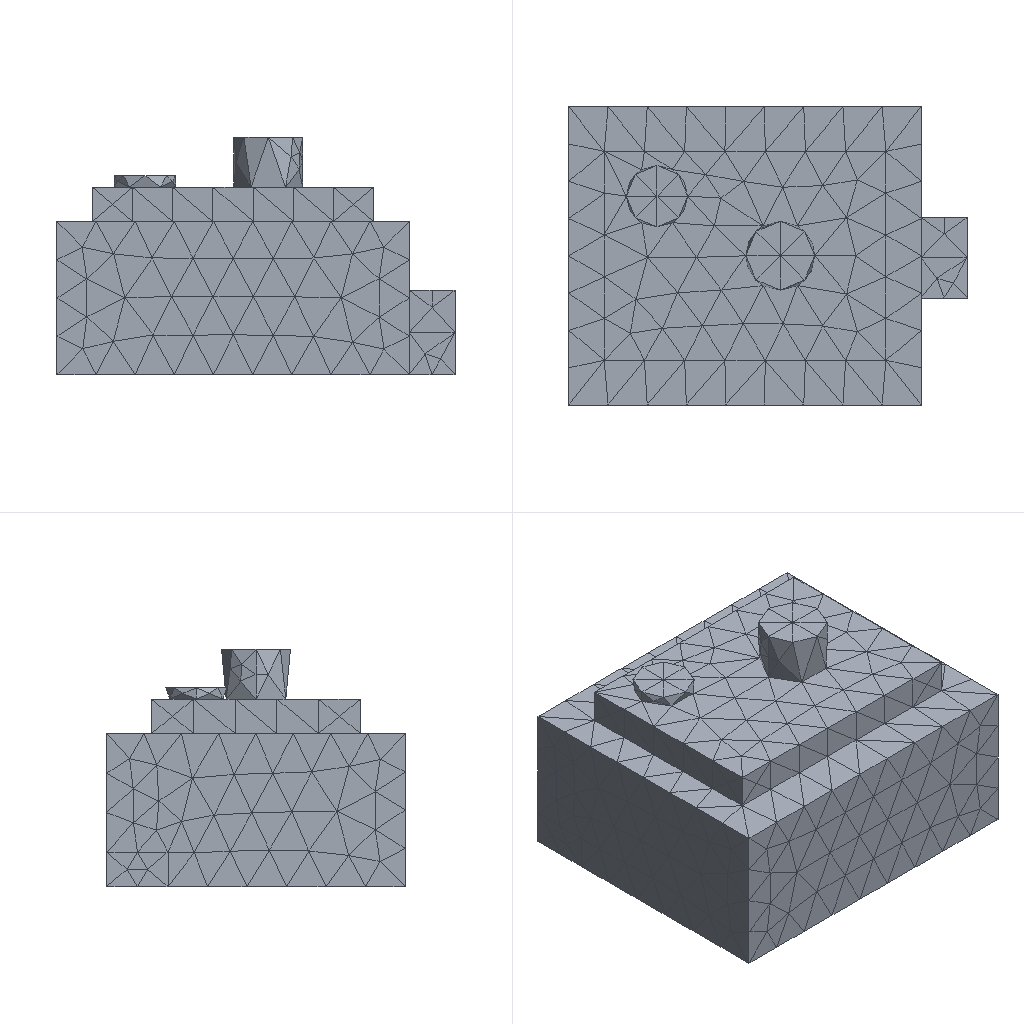Simulation study | ansys mapdl
Set-up summary:
category,name,step,type,value,unit,region
solver,ansys_mapdl
units,mm-N-s-tonne (MPa),,inferred,E=210000 density=
analysis,model,,static
mesh,nodes,,,4234
mesh,elements,,,2509
element_type,SOLID187,,,2509
material,mat 1,,E,210000
material,mat 1,,nu,0.3
load,,model,body load temp,,,all
load,,model,force,"1000 [dir=(0, 0, -1) n=204]",,node list
bc,,model,fixed,"[dofs=UX,UY,UZ n=4625]",,node list
Ansys APDL input file, long lists of numbers shortened:
/COM,ANSYS RELEASE 2026 R1           BUILD 26.1      UP20260202       09:10:16
/PREP7
/NOPR
/TITLE,2
ANTYPE, 0
*IF,_CDRDOFF,EQ,1,THEN     !if solid model was read in
_CDRDOFF=             !reset flag, numoffs already performed
*ELSE              !offset database for the following FE model
NUMOFF,NODE,     4234
NUMOFF,ELEM,     2509
NUMOFF,MAT ,        1
NUMOFF,TYPE,        1
*ENDIF
*SET,_RETURN ,  0.
*SET,_STATUS ,  0.
*SET,_UIQR   ,  204.
*SET,__FLOATPARAMETER__,  4234.
DOF,DELETE
ETBLOCK,        1,        1
(2i9,19a9)
        1      187        0        0        0        0        0        0        0        0        0        0        0        0        0        0        0        0        0        0        0
       -1
NBLOCK,6,SOLID,      4234,      4234
(3i9,6e21.13e3)
        1        0        0-3.0050000000000E+001 3.9000000000000E+001 9.0000000000000E+000
! (4233 more lines like these left out)
N,UNBL,LOC,       -1,
EBLOCK,19,SOLID,      2509,      2509
(19i10)
         1         1         1         1         0         0         0         0        10         0         1       849      1675       664       666      1909      1910      1911      1912
! (5017 more lines like these left out)
        -1
MPTEMP,UNBL, 1, 1,  0.    ,
MPDATA,UNBL, 1,EX  ,       1, 1,  210000.000    ,
MPTEMP,UNBL, 1, 1,  0.    ,
MPDATA,UNBL, 1,NUXY,       1, 1, 0.3    ,
MPTEMP,UNBL, 1, 1,  0.    ,
MPDATA,UNBL, 1,PRXY,       1, 1, 0.3    ,
EXTOPT,ATTR,      0,      0,      0
EXTOPT,ESIZE,  0,  0.
EXTOPT,ACLEAR,      0
TREF,  0.
IRLF,  0
BFUNIF,TEMP,_TINY
ACEL,  0.    ,  0.    ,  0.
OMEGA,  0.    ,  0.    ,  0.
DOMEGA,  0.    ,  0.    ,  0.
CGLOC,  0.    ,  0.    ,  0.
CGOMEGA,  0.    ,  0.    ,  0.
DCGOMG,  0.    ,  0.    ,  0.
KUSE,     0
TIME,  0.
ALPHAD,  0.
BETAD,  0.
DMPRAT,  0.
DMPSTR,  0.
CRPLIM, 0.1    ,   0
CRPLIM,  0.    ,   1
NCNV,     0, 1.000000000E+12,     0,  0.    ,  0.
NEQIT,     0
ERESX,DEFA
DBLOCK,      4625
(i9,a6,2(pg16.9))
        1  UX    0.00000000      0.00000000
! (4624 more lines like these left out)
       -1
FBLOCK,       204
(i9,a6,2(pg16.9))
      795  FZ   -4.90196078      0.00000000
! (203 more lines like these left out)
       -1
/GO
FINISH
Results summary:
result,analysis_type_db,,,static,unstated
result,n_sets,,,1,unstated
result,load_steps[0].set,load_step=1,,1,unstated
result,load_steps[0].substep,load_step=1,,1,unstated
result,load_steps[0].time,load_step=1,,1,unstated
result,load_steps[0].freq,load_step=1,,1,unstated
result,load_steps[0].max_usum,load_step=1,,0.0003245,unstated
result,load_steps[0].max_seqv,load_step=1,,4.598,unstated
result,load_steps[0].reaction_sum.FX,load_step=1,,-5.31841e-12,unstated
result,load_steps[0].reaction_sum.FY,load_step=1,,-8.6402e-12,unstated
result,load_steps[0].reaction_sum.FZ,load_step=1,,1000,unstated
result,load_steps[0].reaction_sum.MX,load_step=1,,0,unstated
result,load_steps[0].reaction_sum.MY,load_step=1,,0,unstated
result,load_steps[0].reaction_sum.MZ,load_step=1,,0,unstated
result,convergence,,,results present for all listed sets,unstated